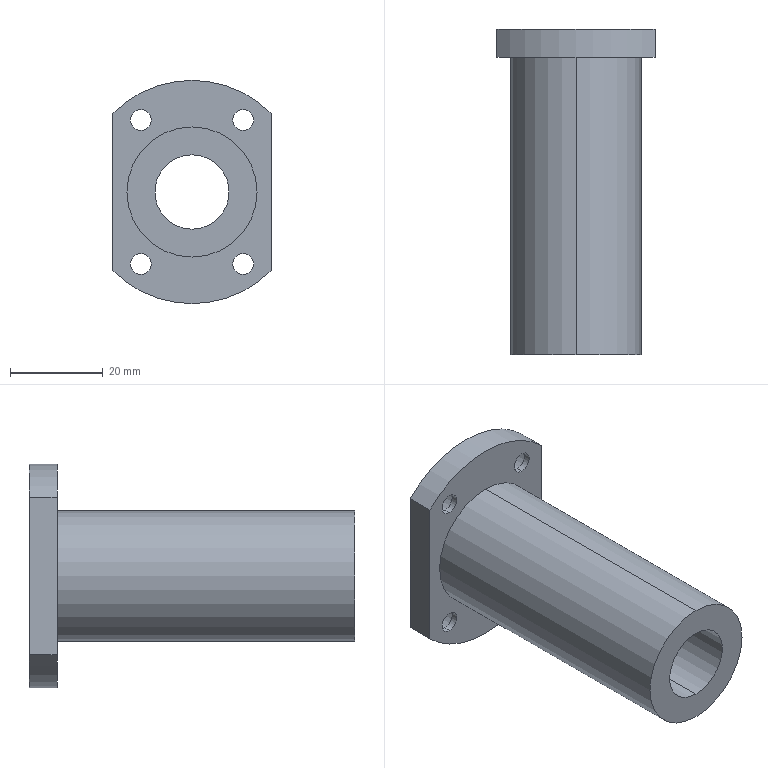Part | SolidWorks | features ICE 3, Extrusion 1, HoleWzd 1 | 1 solid | 32 faces | box 34 x 70 x 48 mm | volume 33217 mm3 | cylinder 23 | plane 9 | commonest cylinder face diameters 4.5 x8 8 x8 48 x3 16 x2 28 x2
STEP:
#1=CARTESIAN_POINT('',(11.,65.4,11.5));
#2=VERTEX_POINT('',#1);
#3=CARTESIAN_POINT('',(11.,65.4,19.5));
#4=VERTEX_POINT('',#3);
#5=CARTESIAN_POINT('',(11.,65.4,15.5));
#6=DIRECTION('',(0.,1.,0.));
#7=DIRECTION('',(0.,0.,1.));
#8=AXIS2_PLACEMENT_3D('',#5,#6,#7);
#9=CIRCLE('',#8,4.);
#10=EDGE_CURVE('',#2,#4,#9,.T.);
#11=ORIENTED_EDGE('',*,*,#10,.F.);
#12=CARTESIAN_POINT('',(11.,70.,11.5));
#13=VERTEX_POINT('',#12);
#14=CARTESIAN_POINT('',(11.,70.,11.5));
#15=DIRECTION('',(0.,1.,0.));
#16=VECTOR('',#15,1000.);
#17=LINE('',#14,#16);
#18=EDGE_CURVE('',#2,#13,#17,.T.);
#19=ORIENTED_EDGE('',*,*,#18,.T.);
#20=CARTESIAN_POINT('',(11.,70.,19.5));
#21=VERTEX_POINT('',#20);
#22=CARTESIAN_POINT('',(11.,70.,15.5));
#23=DIRECTION('',(0.,1.,0.));
#24=DIRECTION('',(0.,0.,1.));
#25=AXIS2_PLACEMENT_3D('',#22,#23,#24);
#26=CIRCLE('',#25,4.);
#27=EDGE_CURVE('',#13,#21,#26,.T.);
#28=ORIENTED_EDGE('',*,*,#27,.T.);
#29=CARTESIAN_POINT('',(11.,70.,19.5));
#30=DIRECTION('',(0.,1.,0.));
#31=VECTOR('',#30,1000.);
#32=LINE('',#29,#31);
#33=EDGE_CURVE('',#4,#21,#32,.T.);
#34=ORIENTED_EDGE('',*,*,#33,.F.);
#35=EDGE_LOOP('',(#11,#19,#28,#34));
#36=FACE_OUTER_BOUND('',#35,.T.);
#37=CARTESIAN_POINT('',(11.,70.,15.5));
#38=DIRECTION('',(0.,1.,0.));
#39=DIRECTION('',(0.,0.,1.));
#40=AXIS2_PLACEMENT_3D('',#37,#38,#39);
#41=CYLINDRICAL_SURFACE('',#40,4.);
#42=ADVANCED_FACE('',(#36),#41,.F.);
#43=CARTESIAN_POINT('',(11.,64.,13.25));
#44=VERTEX_POINT('',#43);
#45=CARTESIAN_POINT('',(11.,64.,17.75));
#46=VERTEX_POINT('',#45);
#47=CARTESIAN_POINT('',(11.,64.,15.5));
#48=DIRECTION('',(0.,1.,0.));
#49=DIRECTION('',(0.,0.,1.));
#50=AXIS2_PLACEMENT_3D('',#47,#48,#49);
#51=CIRCLE('',#50,2.25);
#52=EDGE_CURVE('',#44,#46,#51,.T.);
#53=ORIENTED_EDGE('',*,*,#52,.F.);
#54=CARTESIAN_POINT('',(11.,65.4,13.25));
#55=VERTEX_POINT('',#54);
#56=CARTESIAN_POINT('',(11.,70.,13.25));
#57=DIRECTION('',(0.,1.,0.));
#58=VECTOR('',#57,1000.);
#59=LINE('',#56,#58);
#60=EDGE_CURVE('',#44,#55,#59,.T.);
#61=ORIENTED_EDGE('',*,*,#60,.T.);
#62=CARTESIAN_POINT('',(11.,65.4,17.75));
#63=VERTEX_POINT('',#62);
#64=CARTESIAN_POINT('',(11.,65.4,15.5));
#65=DIRECTION('',(0.,1.,0.));
#66=DIRECTION('',(0.,0.,1.));
#67=AXIS2_PLACEMENT_3D('',#64,#65,#66);
#68=CIRCLE('',#67,2.25);
#69=EDGE_CURVE('',#55,#63,#68,.T.);
#70=ORIENTED_EDGE('',*,*,#69,.T.);
#71=CARTESIAN_POINT('',(11.,70.,17.75));
#72=DIRECTION('',(0.,1.,0.));
#73=VECTOR('',#72,1000.);
#74=LINE('',#71,#73);
#75=EDGE_CURVE('',#46,#63,#74,.T.);
#76=ORIENTED_EDGE('',*,*,#75,.F.);
#77=EDGE_LOOP('',(#53,#61,#70,#76));
#78=FACE_OUTER_BOUND('',#77,.T.);
#79=CARTESIAN_POINT('',(11.,70.,15.5));
#80=DIRECTION('',(0.,1.,0.));
#81=DIRECTION('',(0.,0.,1.));
#82=AXIS2_PLACEMENT_3D('',#79,#80,#81);
#83=CYLINDRICAL_SURFACE('',#82,2.25);
#84=ADVANCED_FACE('',(#78),#83,.F.);
#85=CARTESIAN_POINT('',(-11.,65.4,11.5));
#86=VERTEX_POINT('',#85);
#87=CARTESIAN_POINT('',(-11.,65.4,19.5));
#88=VERTEX_POINT('',#87);
#89=CARTESIAN_POINT('',(-11.,65.4,15.5));
#90=DIRECTION('',(0.,1.,0.));
#91=DIRECTION('',(0.,0.,1.));
#92=AXIS2_PLACEMENT_3D('',#89,#90,#91);
#93=CIRCLE('',#92,4.);
#94=EDGE_CURVE('',#86,#88,#93,.T.);
#95=ORIENTED_EDGE('',*,*,#94,.F.);
#96=CARTESIAN_POINT('',(-11.,70.,11.5));
#97=VERTEX_POINT('',#96);
#98=CARTESIAN_POINT('',(-11.,70.,11.5));
#99=DIRECTION('',(0.,1.,0.));
#100=VECTOR('',#99,1000.);
#101=LINE('',#98,#100);
#102=EDGE_CURVE('',#86,#97,#101,.T.);
#103=ORIENTED_EDGE('',*,*,#102,.T.);
#104=CARTESIAN_POINT('',(-11.,70.,19.5));
#105=VERTEX_POINT('',#104);
#106=CARTESIAN_POINT('',(-11.,70.,15.5));
#107=DIRECTION('',(0.,1.,0.));
#108=DIRECTION('',(0.,0.,1.));
#109=AXIS2_PLACEMENT_3D('',#106,#107,#108);
#110=CIRCLE('',#109,4.);
#111=EDGE_CURVE('',#97,#105,#110,.T.);
#112=ORIENTED_EDGE('',*,*,#111,.T.);
#113=CARTESIAN_POINT('',(-11.,70.,19.5));
#114=DIRECTION('',(0.,1.,0.));
#115=VECTOR('',#114,1000.);
#116=LINE('',#113,#115);
#117=EDGE_CURVE('',#88,#105,#116,.T.);
#118=ORIENTED_EDGE('',*,*,#117,.F.);
#119=EDGE_LOOP('',(#95,#103,#112,#118));
#120=FACE_OUTER_BOUND('',#119,.T.);
#121=CARTESIAN_POINT('',(-11.,70.,15.5));
#122=DIRECTION('',(0.,1.,0.));
#123=DIRECTION('',(0.,0.,1.));
#124=AXIS2_PLACEMENT_3D('',#121,#122,#123);
#125=CYLINDRICAL_SURFACE('',#124,4.);
#126=ADVANCED_FACE('',(#120),#125,.F.);
#127=CARTESIAN_POINT('',(-11.,64.,13.25));
#128=VERTEX_POINT('',#127);
#129=CARTESIAN_POINT('',(-11.,64.,17.75));
#130=VERTEX_POINT('',#129);
#131=CARTESIAN_POINT('',(-11.,64.,15.5));
#132=DIRECTION('',(0.,1.,0.));
#133=DIRECTION('',(0.,0.,1.));
#134=AXIS2_PLACEMENT_3D('',#131,#132,#133);
#135=CIRCLE('',#134,2.25);
#136=EDGE_CURVE('',#128,#130,#135,.T.);
#137=ORIENTED_EDGE('',*,*,#136,.F.);
#138=CARTESIAN_POINT('',(-11.,65.4,13.25));
#139=VERTEX_POINT('',#138);
#140=CARTESIAN_POINT('',(-11.,70.,13.25));
#141=DIRECTION('',(0.,1.,0.));
#142=VECTOR('',#141,1000.);
#143=LINE('',#140,#142);
#144=EDGE_CURVE('',#128,#139,#143,.T.);
#145=ORIENTED_EDGE('',*,*,#144,.T.);
#146=CARTESIAN_POINT('',(-11.,65.4,17.75));
#147=VERTEX_POINT('',#146);
#148=CARTESIAN_POINT('',(-11.,65.4,15.5));
#149=DIRECTION('',(0.,1.,0.));
#150=DIRECTION('',(0.,0.,1.));
#151=AXIS2_PLACEMENT_3D('',#148,#149,#150);
#152=CIRCLE('',#151,2.25);
#153=EDGE_CURVE('',#139,#147,#152,.T.);
#154=ORIENTED_EDGE('',*,*,#153,.T.);
#155=CARTESIAN_POINT('',(-11.,70.,17.75));
#156=DIRECTION('',(0.,1.,0.));
#157=VECTOR('',#156,1000.);
#158=LINE('',#155,#157);
#159=EDGE_CURVE('',#130,#147,#158,.T.);
#160=ORIENTED_EDGE('',*,*,#159,.F.);
#161=EDGE_LOOP('',(#137,#145,#154,#160));
#162=FACE_OUTER_BOUND('',#161,.T.);
#163=CARTESIAN_POINT('',(-11.,70.,15.5));
#164=DIRECTION('',(0.,1.,0.));
#165=DIRECTION('',(0.,0.,1.));
#166=AXIS2_PLACEMENT_3D('',#163,#164,#165);
#167=CYLINDRICAL_SURFACE('',#166,2.25);
#168=ADVANCED_FACE('',(#162),#167,.F.);
#169=CARTESIAN_POINT('',(-11.,65.4,-19.5));
#170=VERTEX_POINT('',#169);
#171=CARTESIAN_POINT('',(-11.,65.4,-11.5));
#172=VERTEX_POINT('',#171);
#173=CARTESIAN_POINT('',(-11.,65.4,-15.5));
#174=DIRECTION('',(0.,1.,0.));
#175=DIRECTION('',(0.,0.,1.));
#176=AXIS2_PLACEMENT_3D('',#173,#174,#175);
#177=CIRCLE('',#176,4.);
#178=EDGE_CURVE('',#170,#172,#177,.T.);
#179=ORIENTED_EDGE('',*,*,#178,.F.);
#180=CARTESIAN_POINT('',(-11.,70.,-19.5));
#181=VERTEX_POINT('',#180);
#182=CARTESIAN_POINT('',(-11.,70.,-19.5));
#183=DIRECTION('',(0.,1.,0.));
#184=VECTOR('',#183,1000.);
#185=LINE('',#182,#184);
#186=EDGE_CURVE('',#170,#181,#185,.T.);
#187=ORIENTED_EDGE('',*,*,#186,.T.);
#188=CARTESIAN_POINT('',(-11.,70.,-11.5));
#189=VERTEX_POINT('',#188);
#190=CARTESIAN_POINT('',(-11.,70.,-15.5));
#191=DIRECTION('',(0.,1.,0.));
#192=DIRECTION('',(0.,0.,1.));
#193=AXIS2_PLACEMENT_3D('',#190,#191,#192);
#194=CIRCLE('',#193,4.);
#195=EDGE_CURVE('',#181,#189,#194,.T.);
#196=ORIENTED_EDGE('',*,*,#195,.T.);
#197=CARTESIAN_POINT('',(-11.,70.,-11.5));
#198=DIRECTION('',(0.,1.,0.));
#199=VECTOR('',#198,1000.);
#200=LINE('',#197,#199);
#201=EDGE_CURVE('',#172,#189,#200,.T.);
#202=ORIENTED_EDGE('',*,*,#201,.F.);
#203=EDGE_LOOP('',(#179,#187,#196,#202));
#204=FACE_OUTER_BOUND('',#203,.T.);
#205=CARTESIAN_POINT('',(-11.,70.,-15.5));
#206=DIRECTION('',(0.,1.,0.));
#207=DIRECTION('',(0.,0.,1.));
#208=AXIS2_PLACEMENT_3D('',#205,#206,#207);
#209=CYLINDRICAL_SURFACE('',#208,4.);
#210=ADVANCED_FACE('',(#204),#209,.F.);
#211=CARTESIAN_POINT('',(-11.,64.,-17.75));
#212=VERTEX_POINT('',#211);
#213=CARTESIAN_POINT('',(-11.,64.,-13.25));
#214=VERTEX_POINT('',#213);
#215=CARTESIAN_POINT('',(-11.,64.,-15.5));
#216=DIRECTION('',(0.,1.,0.));
#217=DIRECTION('',(0.,0.,1.));
#218=AXIS2_PLACEMENT_3D('',#215,#216,#217);
#219=CIRCLE('',#218,2.25);
#220=EDGE_CURVE('',#212,#214,#219,.T.);
#221=ORIENTED_EDGE('',*,*,#220,.F.);
#222=CARTESIAN_POINT('',(-11.,65.4,-17.75));
#223=VERTEX_POINT('',#222);
#224=CARTESIAN_POINT('',(-11.,70.,-17.75));
#225=DIRECTION('',(0.,1.,0.));
#226=VECTOR('',#225,1000.);
#227=LINE('',#224,#226);
#228=EDGE_CURVE('',#212,#223,#227,.T.);
#229=ORIENTED_EDGE('',*,*,#228,.T.);
#230=CARTESIAN_POINT('',(-11.,65.4,-13.25));
#231=VERTEX_POINT('',#230);
#232=CARTESIAN_POINT('',(-11.,65.4,-15.5));
#233=DIRECTION('',(0.,1.,0.));
#234=DIRECTION('',(0.,0.,1.));
#235=AXIS2_PLACEMENT_3D('',#232,#233,#234);
#236=CIRCLE('',#235,2.25);
#237=EDGE_CURVE('',#223,#231,#236,.T.);
#238=ORIENTED_EDGE('',*,*,#237,.T.);
#239=CARTESIAN_POINT('',(-11.,70.,-13.25));
#240=DIRECTION('',(0.,1.,0.));
#241=VECTOR('',#240,1000.);
#242=LINE('',#239,#241);
#243=EDGE_CURVE('',#214,#231,#242,.T.);
#244=ORIENTED_EDGE('',*,*,#243,.F.);
#245=EDGE_LOOP('',(#221,#229,#238,#244));
#246=FACE_OUTER_BOUND('',#245,.T.);
#247=CARTESIAN_POINT('',(-11.,70.,-15.5));
#248=DIRECTION('',(0.,1.,0.));
#249=DIRECTION('',(0.,0.,1.));
#250=AXIS2_PLACEMENT_3D('',#247,#248,#249);
#251=CYLINDRICAL_SURFACE('',#250,2.25);
#252=ADVANCED_FACE('',(#246),#251,.F.);
#253=CARTESIAN_POINT('',(11.,65.4,-19.5));
#254=VERTEX_POINT('',#253);
#255=CARTESIAN_POINT('',(11.,65.4,-11.5));
#256=VERTEX_POINT('',#255);
#257=CARTESIAN_POINT('',(11.,65.4,-15.5));
#258=DIRECTION('',(0.,1.,0.));
#259=DIRECTION('',(0.,0.,1.));
#260=AXIS2_PLACEMENT_3D('',#257,#258,#259);
#261=CIRCLE('',#260,4.);
#262=EDGE_CURVE('',#254,#256,#261,.T.);
#263=ORIENTED_EDGE('',*,*,#262,.F.);
#264=CARTESIAN_POINT('',(11.,70.,-19.5));
#265=VERTEX_POINT('',#264);
#266=CARTESIAN_POINT('',(11.,70.,-19.5));
#267=DIRECTION('',(0.,1.,0.));
#268=VECTOR('',#267,1000.);
#269=LINE('',#266,#268);
#270=EDGE_CURVE('',#254,#265,#269,.T.);
#271=ORIENTED_EDGE('',*,*,#270,.T.);
#272=CARTESIAN_POINT('',(11.,70.,-11.5));
#273=VERTEX_POINT('',#272);
#274=CARTESIAN_POINT('',(11.,70.,-15.5));
#275=DIRECTION('',(0.,1.,0.));
#276=DIRECTION('',(0.,0.,1.));
#277=AXIS2_PLACEMENT_3D('',#274,#275,#276);
#278=CIRCLE('',#277,4.);
#279=EDGE_CURVE('',#265,#273,#278,.T.);
#280=ORIENTED_EDGE('',*,*,#279,.T.);
#281=CARTESIAN_POINT('',(11.,70.,-11.5));
#282=DIRECTION('',(0.,1.,0.));
#283=VECTOR('',#282,1000.);
#284=LINE('',#281,#283);
#285=EDGE_CURVE('',#256,#273,#284,.T.);
#286=ORIENTED_EDGE('',*,*,#285,.F.);
#287=EDGE_LOOP('',(#263,#271,#280,#286));
#288=FACE_OUTER_BOUND('',#287,.T.);
#289=CARTESIAN_POINT('',(11.,70.,-15.5));
#290=DIRECTION('',(0.,1.,0.));
#291=DIRECTION('',(0.,0.,1.));
#292=AXIS2_PLACEMENT_3D('',#289,#290,#291);
#293=CYLINDRICAL_SURFACE('',#292,4.);
#294=ADVANCED_FACE('',(#288),#293,.F.);
#295=CARTESIAN_POINT('',(11.,64.,-17.75));
#296=VERTEX_POINT('',#295);
#297=CARTESIAN_POINT('',(11.,64.,-13.25));
#298=VERTEX_POINT('',#297);
#299=CARTESIAN_POINT('',(11.,64.,-15.5));
#300=DIRECTION('',(0.,1.,0.));
#301=DIRECTION('',(0.,0.,1.));
#302=AXIS2_PLACEMENT_3D('',#299,#300,#301);
#303=CIRCLE('',#302,2.25);
#304=EDGE_CURVE('',#296,#298,#303,.T.);
#305=ORIENTED_EDGE('',*,*,#304,.F.);
#306=CARTESIAN_POINT('',(11.,65.4,-17.75));
#307=VERTEX_POINT('',#306);
#308=CARTESIAN_POINT('',(11.,70.,-17.75));
#309=DIRECTION('',(0.,1.,0.));
#310=VECTOR('',#309,1000.);
#311=LINE('',#308,#310);
#312=EDGE_CURVE('',#296,#307,#311,.T.);
#313=ORIENTED_EDGE('',*,*,#312,.T.);
#314=CARTESIAN_POINT('',(11.,65.4,-13.25));
#315=VERTEX_POINT('',#314);
#316=CARTESIAN_POINT('',(11.,65.4,-15.5));
#317=DIRECTION('',(0.,1.,0.));
#318=DIRECTION('',(0.,0.,1.));
#319=AXIS2_PLACEMENT_3D('',#316,#317,#318);
#320=CIRCLE('',#319,2.25);
#321=EDGE_CURVE('',#307,#315,#320,.T.);
#322=ORIENTED_EDGE('',*,*,#321,.T.);
#323=CARTESIAN_POINT('',(11.,70.,-13.25));
#324=DIRECTION('',(0.,1.,0.));
#325=VECTOR('',#324,1000.);
#326=LINE('',#323,#325);
#327=EDGE_CURVE('',#298,#315,#326,.T.);
#328=ORIENTED_EDGE('',*,*,#327,.F.);
#329=EDGE_LOOP('',(#305,#313,#322,#328));
#330=FACE_OUTER_BOUND('',#329,.T.);
#331=CARTESIAN_POINT('',(11.,70.,-15.5));
#332=DIRECTION('',(0.,1.,0.));
#333=DIRECTION('',(0.,0.,1.));
#334=AXIS2_PLACEMENT_3D('',#331,#332,#333);
#335=CYLINDRICAL_SURFACE('',#334,2.25);
#336=ADVANCED_FACE('',(#330),#335,.F.);
#337=CARTESIAN_POINT('',(0.,70.,8.));
#338=VERTEX_POINT('',#337);
#339=CARTESIAN_POINT('',(0.,70.,-8.));
#340=VERTEX_POINT('',#339);
#341=CARTESIAN_POINT('',(0.,70.,0.));
#342=DIRECTION('',(0.,-1.,0.));
#343=DIRECTION('',(0.,0.,-1.));
#344=AXIS2_PLACEMENT_3D('',#341,#342,#343);
#345=CIRCLE('',#344,8.);
#346=EDGE_CURVE('',#338,#340,#345,.T.);
#347=ORIENTED_EDGE('',*,*,#346,.F.);
#348=CARTESIAN_POINT('',(0.,0.,8.));
#349=VERTEX_POINT('',#348);
#350=CARTESIAN_POINT('',(0.,70.,8.));
#351=DIRECTION('',(0.,-1.,0.));
#352=VECTOR('',#351,1000.);
#353=LINE('',#350,#352);
#354=EDGE_CURVE('',#338,#349,#353,.T.);
#355=ORIENTED_EDGE('',*,*,#354,.T.);
#356=CARTESIAN_POINT('',(0.,0.,-8.));
#357=VERTEX_POINT('',#356);
#358=CARTESIAN_POINT('',(0.,0.,0.));
#359=DIRECTION('',(0.,-1.,0.));
#360=DIRECTION('',(0.,0.,-1.));
#361=AXIS2_PLACEMENT_3D('',#358,#359,#360);
#362=CIRCLE('',#361,8.);
#363=EDGE_CURVE('',#349,#357,#362,.T.);
#364=ORIENTED_EDGE('',*,*,#363,.T.);
#365=CARTESIAN_POINT('',(0.,70.,-8.));
#366=DIRECTION('',(0.,-1.,0.));
#367=VECTOR('',#366,1000.);
#368=LINE('',#365,#367);
#369=EDGE_CURVE('',#340,#357,#368,.T.);
#370=ORIENTED_EDGE('',*,*,#369,.F.);
#371=EDGE_LOOP('',(#347,#355,#364,#370));
#372=FACE_OUTER_BOUND('',#371,.T.);
#373=CARTESIAN_POINT('',(0.,70.,0.));
#374=DIRECTION('',(0.,-1.,0.));
#375=DIRECTION('',(0.,0.,-1.));
#376=AXIS2_PLACEMENT_3D('',#373,#374,#375);
#377=CYLINDRICAL_SURFACE('',#376,8.);
#378=ADVANCED_FACE('',(#372),#377,.F.);
#379=CARTESIAN_POINT('',(0.,64.,14.));
#380=VERTEX_POINT('',#379);
#381=CARTESIAN_POINT('',(0.,64.,-14.));
#382=VERTEX_POINT('',#381);
#383=CARTESIAN_POINT('',(0.,64.,0.));
#384=DIRECTION('',(0.,1.,0.));
#385=DIRECTION('',(0.,0.,1.));
#386=AXIS2_PLACEMENT_3D('',#383,#384,#385);
#387=CIRCLE('',#386,14.);
#388=EDGE_CURVE('',#380,#382,#387,.T.);
#389=ORIENTED_EDGE('',*,*,#388,.F.);
#390=CARTESIAN_POINT('',(0.,0.,14.));
#391=VERTEX_POINT('',#390);
#392=CARTESIAN_POINT('',(0.,64.,14.));
#393=DIRECTION('',(0.,-1.,0.));
#394=VECTOR('',#393,1000.);
#395=LINE('',#392,#394);
#396=EDGE_CURVE('',#380,#391,#395,.T.);
#397=ORIENTED_EDGE('',*,*,#396,.T.);
#398=CARTESIAN_POINT('',(0.,0.,-14.));
#399=VERTEX_POINT('',#398);
#400=CARTESIAN_POINT('',(0.,0.,0.));
#401=DIRECTION('',(0.,1.,0.));
#402=DIRECTION('',(0.,0.,1.));
#403=AXIS2_PLACEMENT_3D('',#400,#401,#402);
#404=CIRCLE('',#403,14.);
#405=EDGE_CURVE('',#391,#399,#404,.T.);
#406=ORIENTED_EDGE('',*,*,#405,.T.);
#407=CARTESIAN_POINT('',(0.,64.,-14.));
#408=DIRECTION('',(0.,-1.,0.));
#409=VECTOR('',#408,1000.);
#410=LINE('',#407,#409);
#411=EDGE_CURVE('',#382,#399,#410,.T.);
#412=ORIENTED_EDGE('',*,*,#411,.F.);
#413=EDGE_LOOP('',(#389,#397,#406,#412));
#414=FACE_OUTER_BOUND('',#413,.T.);
#415=CARTESIAN_POINT('',(0.,64.,0.));
#416=DIRECTION('',(0.,-1.,0.));
#417=DIRECTION('',(0.,0.,-1.));
#418=AXIS2_PLACEMENT_3D('',#415,#416,#417);
#419=CYLINDRICAL_SURFACE('',#418,14.);
#420=ADVANCED_FACE('',(#414),#419,.T.);
#421=CARTESIAN_POINT('',(0.,70.,-24.));
#422=VERTEX_POINT('',#421);
#423=CARTESIAN_POINT('',(-17.,70.,-16.941));
#424=VERTEX_POINT('',#423);
#425=CARTESIAN_POINT('',(0.,70.,0.));
#426=DIRECTION('',(0.,1.,0.));
#427=DIRECTION('',(0.,0.,1.));
#428=AXIS2_PLACEMENT_3D('',#425,#426,#427);
#429=CIRCLE('',#428,24.);
#430=EDGE_CURVE('',#422,#424,#429,.T.);
#431=ORIENTED_EDGE('',*,*,#430,.F.);
#432=CARTESIAN_POINT('',(0.,64.,-24.));
#433=VERTEX_POINT('',#432);
#434=CARTESIAN_POINT('',(0.,70.,-24.));
#435=DIRECTION('',(0.,-1.,0.));
#436=VECTOR('',#435,1000.);
#437=LINE('',#434,#436);
#438=EDGE_CURVE('',#422,#433,#437,.T.);
#439=ORIENTED_EDGE('',*,*,#438,.T.);
#440=CARTESIAN_POINT('',(-17.,64.,-16.941));
#441=VERTEX_POINT('',#440);
#442=CARTESIAN_POINT('',(0.,64.,0.));
#443=DIRECTION('',(0.,1.,0.));
#444=DIRECTION('',(0.,0.,1.));
#445=AXIS2_PLACEMENT_3D('',#442,#443,#444);
#446=CIRCLE('',#445,24.);
#447=EDGE_CURVE('',#433,#441,#446,.T.);
#448=ORIENTED_EDGE('',*,*,#447,.T.);
#449=CARTESIAN_POINT('',(-17.,64.,-16.941));
#450=DIRECTION('',(0.,1.,0.));
#451=VECTOR('',#450,1000.);
#452=LINE('',#449,#451);
#453=EDGE_CURVE('',#441,#424,#452,.T.);
#454=ORIENTED_EDGE('',*,*,#453,.T.);
#455=EDGE_LOOP('',(#431,#439,#448,#454));
#456=FACE_OUTER_BOUND('',#455,.T.);
#457=CARTESIAN_POINT('',(0.,70.,0.));
#458=DIRECTION('',(0.,-1.,0.));
#459=DIRECTION('',(0.,0.,-1.));
#460=AXIS2_PLACEMENT_3D('',#457,#458,#459);
#461=CYLINDRICAL_SURFACE('',#460,24.);
#462=ADVANCED_FACE('',(#456),#461,.T.);
#463=CARTESIAN_POINT('',(11.,64.,15.5));
#464=DIRECTION('',(0.,1.,0.));
#465=DIRECTION('',(0.,0.,1.));
#466=AXIS2_PLACEMENT_3D('',#463,#464,#465);
#467=CIRCLE('',#466,2.25);
#468=EDGE_CURVE('',#46,#44,#467,.T.);
#469=ORIENTED_EDGE('',*,*,#468,.T.);
#470=ORIENTED_EDGE('',*,*,#52,.T.);
#471=EDGE_LOOP('',(#469,#470));
#472=FACE_BOUND('',#471,.T.);
#473=CARTESIAN_POINT('',(-11.,64.,15.5));
#474=DIRECTION('',(0.,1.,0.));
#475=DIRECTION('',(0.,0.,1.));
#476=AXIS2_PLACEMENT_3D('',#473,#474,#475);
#477=CIRCLE('',#476,2.25);
#478=EDGE_CURVE('',#130,#128,#477,.T.);
#479=ORIENTED_EDGE('',*,*,#478,.T.);
#480=ORIENTED_EDGE('',*,*,#136,.T.);
#481=EDGE_LOOP('',(#479,#480));
#482=FACE_BOUND('',#481,.T.);
#483=CARTESIAN_POINT('',(-11.,64.,-15.5));
#484=DIRECTION('',(0.,1.,0.));
#485=DIRECTION('',(0.,0.,1.));
#486=AXIS2_PLACEMENT_3D('',#483,#484,#485);
#487=CIRCLE('',#486,2.25);
#488=EDGE_CURVE('',#214,#212,#487,.T.);
#489=ORIENTED_EDGE('',*,*,#488,.T.);
#490=ORIENTED_EDGE('',*,*,#220,.T.);
#491=EDGE_LOOP('',(#489,#490));
#492=FACE_BOUND('',#491,.T.);
#493=CARTESIAN_POINT('',(11.,64.,-15.5));
#494=DIRECTION('',(0.,1.,0.));
#495=DIRECTION('',(0.,0.,1.));
#496=AXIS2_PLACEMENT_3D('',#493,#494,#495);
#497=CIRCLE('',#496,2.25);
#498=EDGE_CURVE('',#298,#296,#497,.T.);
#499=ORIENTED_EDGE('',*,*,#498,.T.);
#500=ORIENTED_EDGE('',*,*,#304,.T.);
#501=EDGE_LOOP('',(#499,#500));
#502=FACE_BOUND('',#501,.T.);
#503=CARTESIAN_POINT('',(0.,64.,0.));
#504=DIRECTION('',(0.,1.,0.));
#505=DIRECTION('',(0.,0.,1.));
#506=AXIS2_PLACEMENT_3D('',#503,#504,#505);
#507=CIRCLE('',#506,14.);
#508=EDGE_CURVE('',#382,#380,#507,.T.);
#509=ORIENTED_EDGE('',*,*,#508,.T.);
#510=ORIENTED_EDGE('',*,*,#388,.T.);
#511=EDGE_LOOP('',(#509,#510));
#512=FACE_BOUND('',#511,.T.);
#513=CARTESIAN_POINT('',(17.,64.,16.941));
#514=VERTEX_POINT('',#513);
#515=CARTESIAN_POINT('',(17.,64.,-16.941));
#516=VERTEX_POINT('',#515);
#517=CARTESIAN_POINT('',(17.,64.,-16.941));
#518=DIRECTION('',(0.,0.,-1.));
#519=VECTOR('',#518,1000.);
#520=LINE('',#517,#519);
#521=EDGE_CURVE('',#514,#516,#520,.T.);
#522=ORIENTED_EDGE('',*,*,#521,.F.);
#523=CARTESIAN_POINT('',(-17.,64.,16.941));
#524=VERTEX_POINT('',#523);
#525=CARTESIAN_POINT('',(0.,64.,0.));
#526=DIRECTION('',(0.,1.,0.));
#527=DIRECTION('',(0.,0.,1.));
#528=AXIS2_PLACEMENT_3D('',#525,#526,#527);
#529=CIRCLE('',#528,24.);
#530=EDGE_CURVE('',#524,#514,#529,.T.);
#531=ORIENTED_EDGE('',*,*,#530,.F.);
#532=CARTESIAN_POINT('',(-17.,64.,-16.941));
#533=DIRECTION('',(0.,0.,1.));
#534=VECTOR('',#533,1000.);
#535=LINE('',#532,#534);
#536=EDGE_CURVE('',#441,#524,#535,.T.);
#537=ORIENTED_EDGE('',*,*,#536,.F.);
#538=ORIENTED_EDGE('',*,*,#447,.F.);
#539=CARTESIAN_POINT('',(0.,64.,0.));
#540=DIRECTION('',(0.,1.,0.));
#541=DIRECTION('',(0.,0.,1.));
#542=AXIS2_PLACEMENT_3D('',#539,#540,#541);
#543=CIRCLE('',#542,24.);
#544=EDGE_CURVE('',#516,#433,#543,.T.);
#545=ORIENTED_EDGE('',*,*,#544,.F.);
#546=EDGE_LOOP('',(#522,#531,#537,#538,#545));
#547=FACE_OUTER_BOUND('',#546,.T.);
#548=CARTESIAN_POINT('',(0.,64.,0.));
#549=DIRECTION('',(0.,1.,0.));
#550=DIRECTION('',(0.,0.,1.));
#551=AXIS2_PLACEMENT_3D('',#548,#549,#550);
#552=PLANE('',#551);
#553=ADVANCED_FACE('',(#472,#482,#492,#502,#512,#547),#552,.F.);
#554=CARTESIAN_POINT('',(17.,70.,16.941));
#555=VERTEX_POINT('',#554);
#556=CARTESIAN_POINT('',(17.,64.,16.941));
#557=DIRECTION('',(0.,1.,0.));
#558=VECTOR('',#557,1000.);
#559=LINE('',#556,#558);
#560=EDGE_CURVE('',#514,#555,#559,.T.);
#561=ORIENTED_EDGE('',*,*,#560,.T.);
#562=CARTESIAN_POINT('',(-17.,70.,16.941));
#563=VERTEX_POINT('',#562);
#564=CARTESIAN_POINT('',(0.,70.,0.));
#565=DIRECTION('',(0.,1.,0.));
#566=DIRECTION('',(0.,0.,1.));
#567=AXIS2_PLACEMENT_3D('',#564,#565,#566);
#568=CIRCLE('',#567,24.);
#569=EDGE_CURVE('',#563,#555,#568,.T.);
#570=ORIENTED_EDGE('',*,*,#569,.F.);
#571=CARTESIAN_POINT('',(-17.,64.,16.941));
#572=DIRECTION('',(0.,1.,0.));
#573=VECTOR('',#572,1000.);
#574=LINE('',#571,#573);
#575=EDGE_CURVE('',#524,#563,#574,.T.);
#576=ORIENTED_EDGE('',*,*,#575,.F.);
#577=ORIENTED_EDGE('',*,*,#530,.T.);
#578=EDGE_LOOP('',(#561,#570,#576,#577));
#579=FACE_OUTER_BOUND('',#578,.T.);
#580=CARTESIAN_POINT('',(0.,70.,0.));
#581=DIRECTION('',(0.,-1.,0.));
#582=DIRECTION('',(0.,0.,-1.));
#583=AXIS2_PLACEMENT_3D('',#580,#581,#582);
#584=CYLINDRICAL_SURFACE('',#583,24.);
#585=ADVANCED_FACE('',(#579),#584,.T.);
#586=ORIENTED_EDGE('',*,*,#438,.F.);
#587=CARTESIAN_POINT('',(17.,70.,-16.941));
#588=VERTEX_POINT('',#587);
#589=CARTESIAN_POINT('',(0.,70.,0.));
#590=DIRECTION('',(0.,1.,0.));
#591=DIRECTION('',(0.,0.,1.));
#592=AXIS2_PLACEMENT_3D('',#589,#590,#591);
#593=CIRCLE('',#592,24.);
#594=EDGE_CURVE('',#588,#422,#593,.T.);
#595=ORIENTED_EDGE('',*,*,#594,.F.);
#596=CARTESIAN_POINT('',(17.,64.,-16.941));
#597=DIRECTION('',(0.,1.,0.));
#598=VECTOR('',#597,1000.);
#599=LINE('',#596,#598);
#600=EDGE_CURVE('',#516,#588,#599,.T.);
#601=ORIENTED_EDGE('',*,*,#600,.F.);
#602=ORIENTED_EDGE('',*,*,#544,.T.);
#603=EDGE_LOOP('',(#586,#595,#601,#602));
#604=FACE_OUTER_BOUND('',#603,.T.);
#605=CARTESIAN_POINT('',(0.,70.,0.));
#606=DIRECTION('',(0.,-1.,0.));
#607=DIRECTION('',(0.,0.,-1.));
#608=AXIS2_PLACEMENT_3D('',#605,#606,#607);
#609=CYLINDRICAL_SURFACE('',#608,24.);
#610=ADVANCED_FACE('',(#604),#609,.T.);
#611=CARTESIAN_POINT('',(11.,70.,15.5));
#612=DIRECTION('',(0.,1.,0.));
#613=DIRECTION('',(0.,0.,1.));
#614=AXIS2_PLACEMENT_3D('',#611,#612,#613);
#615=CIRCLE('',#614,4.);
#616=EDGE_CURVE('',#21,#13,#615,.T.);
#617=ORIENTED_EDGE('',*,*,#616,.F.);
#618=ORIENTED_EDGE('',*,*,#27,.F.);
#619=EDGE_LOOP('',(#617,#618));
#620=FACE_BOUND('',#619,.T.);
#621=CARTESIAN_POINT('',(-11.,70.,15.5));
#622=DIRECTION('',(0.,1.,0.));
#623=DIRECTION('',(0.,0.,1.));
#624=AXIS2_PLACEMENT_3D('',#621,#622,#623);
#625=CIRCLE('',#624,4.);
#626=EDGE_CURVE('',#105,#97,#625,.T.);
#627=ORIENTED_EDGE('',*,*,#626,.F.);
#628=ORIENTED_EDGE('',*,*,#111,.F.);
#629=EDGE_LOOP('',(#627,#628));
#630=FACE_BOUND('',#629,.T.);
#631=CARTESIAN_POINT('',(-11.,70.,-15.5));
#632=DIRECTION('',(0.,1.,0.));
#633=DIRECTION('',(0.,0.,1.));
#634=AXIS2_PLACEMENT_3D('',#631,#632,#633);
#635=CIRCLE('',#634,4.);
#636=EDGE_CURVE('',#189,#181,#635,.T.);
#637=ORIENTED_EDGE('',*,*,#636,.F.);
#638=ORIENTED_EDGE('',*,*,#195,.F.);
#639=EDGE_LOOP('',(#637,#638));
#640=FACE_BOUND('',#639,.T.);
#641=CARTESIAN_POINT('',(11.,70.,-15.5));
#642=DIRECTION('',(0.,1.,0.));
#643=DIRECTION('',(0.,0.,1.));
#644=AXIS2_PLACEMENT_3D('',#641,#642,#643);
#645=CIRCLE('',#644,4.);
#646=EDGE_CURVE('',#273,#265,#645,.T.);
#647=ORIENTED_EDGE('',*,*,#646,.F.);
#648=ORIENTED_EDGE('',*,*,#279,.F.);
#649=EDGE_LOOP('',(#647,#648));
#650=FACE_BOUND('',#649,.T.);
#651=CARTESIAN_POINT('',(0.,70.,0.));
#652=DIRECTION('',(0.,-1.,0.));
#653=DIRECTION('',(0.,0.,-1.));
#654=AXIS2_PLACEMENT_3D('',#651,#652,#653);
#655=CIRCLE('',#654,8.);
#656=EDGE_CURVE('',#340,#338,#655,.T.);
#657=ORIENTED_EDGE('',*,*,#656,.T.);
#658=ORIENTED_EDGE('',*,*,#346,.T.);
#659=EDGE_LOOP('',(#657,#658));
#660=FACE_BOUND('',#659,.T.);
#661=ORIENTED_EDGE('',*,*,#569,.T.);
#662=CARTESIAN_POINT('',(17.,70.,-16.941));
#663=DIRECTION('',(0.,0.,-1.));
#664=VECTOR('',#663,1000.);
#665=LINE('',#662,#664);
#666=EDGE_CURVE('',#555,#588,#665,.T.);
#667=ORIENTED_EDGE('',*,*,#666,.T.);
#668=ORIENTED_EDGE('',*,*,#594,.T.);
#669=ORIENTED_EDGE('',*,*,#430,.T.);
#670=CARTESIAN_POINT('',(-17.,70.,-16.941));
#671=DIRECTION('',(0.,0.,1.));
#672=VECTOR('',#671,1000.);
#673=LINE('',#670,#672);
#674=EDGE_CURVE('',#424,#563,#673,.T.);
#675=ORIENTED_EDGE('',*,*,#674,.T.);
#676=EDGE_LOOP('',(#661,#667,#668,#669,#675));
#677=FACE_OUTER_BOUND('',#676,.T.);
#678=CARTESIAN_POINT('',(0.,70.,0.));
#679=DIRECTION('',(0.,1.,0.));
#680=DIRECTION('',(0.,0.,1.));
#681=AXIS2_PLACEMENT_3D('',#678,#679,#680);
#682=PLANE('',#681);
#683=ADVANCED_FACE('',(#620,#630,#640,#650,#660,#677),#682,.T.);
#684=ORIENTED_EDGE('',*,*,#396,.F.);
#685=ORIENTED_EDGE('',*,*,#508,.F.);
#686=ORIENTED_EDGE('',*,*,#411,.T.);
#687=CARTESIAN_POINT('',(0.,0.,0.));
#688=DIRECTION('',(0.,1.,0.));
#689=DIRECTION('',(0.,0.,1.));
#690=AXIS2_PLACEMENT_3D('',#687,#688,#689);
#691=CIRCLE('',#690,14.);
#692=EDGE_CURVE('',#399,#391,#691,.T.);
#693=ORIENTED_EDGE('',*,*,#692,.T.);
#694=EDGE_LOOP('',(#684,#685,#686,#693));
#695=FACE_OUTER_BOUND('',#694,.T.);
#696=CARTESIAN_POINT('',(0.,64.,0.));
#697=DIRECTION('',(0.,-1.,0.));
#698=DIRECTION('',(0.,0.,-1.));
#699=AXIS2_PLACEMENT_3D('',#696,#697,#698);
#700=CYLINDRICAL_SURFACE('',#699,14.);
#701=ADVANCED_FACE('',(#695),#700,.T.);
#702=CARTESIAN_POINT('',(0.,0.,0.));
#703=DIRECTION('',(0.,-1.,0.));
#704=DIRECTION('',(0.,0.,-1.));
#705=AXIS2_PLACEMENT_3D('',#702,#703,#704);
#706=CIRCLE('',#705,8.);
#707=EDGE_CURVE('',#357,#349,#706,.T.);
#708=ORIENTED_EDGE('',*,*,#707,.F.);
#709=ORIENTED_EDGE('',*,*,#363,.F.);
#710=EDGE_LOOP('',(#708,#709));
#711=FACE_BOUND('',#710,.T.);
#712=ORIENTED_EDGE('',*,*,#692,.F.);
#713=ORIENTED_EDGE('',*,*,#405,.F.);
#714=EDGE_LOOP('',(#712,#713));
#715=FACE_OUTER_BOUND('',#714,.T.);
#716=CARTESIAN_POINT('',(0.,0.,0.));
#717=DIRECTION('',(0.,1.,0.));
#718=DIRECTION('',(0.,0.,1.));
#719=AXIS2_PLACEMENT_3D('',#716,#717,#718);
#720=PLANE('',#719);
#721=ADVANCED_FACE('',(#711,#715),#720,.F.);
#722=ORIENTED_EDGE('',*,*,#674,.F.);
#723=ORIENTED_EDGE('',*,*,#453,.F.);
#724=ORIENTED_EDGE('',*,*,#536,.T.);
#725=ORIENTED_EDGE('',*,*,#575,.T.);
#726=EDGE_LOOP('',(#722,#723,#724,#725));
#727=FACE_OUTER_BOUND('',#726,.T.);
#728=CARTESIAN_POINT('',(-17.,64.,-16.941));
#729=DIRECTION('',(-1.,0.,0.));
#730=DIRECTION('',(0.,0.,1.));
#731=AXIS2_PLACEMENT_3D('',#728,#729,#730);
#732=PLANE('',#731);
#733=ADVANCED_FACE('',(#727),#732,.T.);
#734=ORIENTED_EDGE('',*,*,#666,.F.);
#735=ORIENTED_EDGE('',*,*,#560,.F.);
#736=ORIENTED_EDGE('',*,*,#521,.T.);
#737=ORIENTED_EDGE('',*,*,#600,.T.);
#738=EDGE_LOOP('',(#734,#735,#736,#737));
#739=FACE_OUTER_BOUND('',#738,.T.);
#740=CARTESIAN_POINT('',(17.,64.,-16.941));
#741=DIRECTION('',(1.,0.,0.));
#742=DIRECTION('',(0.,0.,-1.));
#743=AXIS2_PLACEMENT_3D('',#740,#741,#742);
#744=PLANE('',#743);
#745=ADVANCED_FACE('',(#739),#744,.T.);
#746=ORIENTED_EDGE('',*,*,#354,.F.);
#747=ORIENTED_EDGE('',*,*,#656,.F.);
#748=ORIENTED_EDGE('',*,*,#369,.T.);
#749=ORIENTED_EDGE('',*,*,#707,.T.);
#750=EDGE_LOOP('',(#746,#747,#748,#749));
#751=FACE_OUTER_BOUND('',#750,.T.);
#752=CARTESIAN_POINT('',(0.,70.,0.));
#753=DIRECTION('',(0.,-1.,0.));
#754=DIRECTION('',(0.,0.,-1.));
#755=AXIS2_PLACEMENT_3D('',#752,#753,#754);
#756=CYLINDRICAL_SURFACE('',#755,8.);
#757=ADVANCED_FACE('',(#751),#756,.F.);
#758=ORIENTED_EDGE('',*,*,#312,.F.);
#759=ORIENTED_EDGE('',*,*,#498,.F.);
#760=ORIENTED_EDGE('',*,*,#327,.T.);
#761=CARTESIAN_POINT('',(11.,65.4,-15.5));
#762=DIRECTION('',(0.,1.,0.));
#763=DIRECTION('',(0.,0.,1.));
#764=AXIS2_PLACEMENT_3D('',#761,#762,#763);
#765=CIRCLE('',#764,2.25);
#766=EDGE_CURVE('',#315,#307,#765,.T.);
#767=ORIENTED_EDGE('',*,*,#766,.T.);
#768=EDGE_LOOP('',(#758,#759,#760,#767));
#769=FACE_OUTER_BOUND('',#768,.T.);
#770=CARTESIAN_POINT('',(11.,70.,-15.5));
#771=DIRECTION('',(0.,1.,0.));
#772=DIRECTION('',(0.,0.,1.));
#773=AXIS2_PLACEMENT_3D('',#770,#771,#772);
#774=CYLINDRICAL_SURFACE('',#773,2.25);
#775=ADVANCED_FACE('',(#769),#774,.F.);
#776=ORIENTED_EDGE('',*,*,#766,.F.);
#777=ORIENTED_EDGE('',*,*,#321,.F.);
#778=EDGE_LOOP('',(#776,#777));
#779=FACE_BOUND('',#778,.T.);
#780=CARTESIAN_POINT('',(11.,65.4,-15.5));
#781=DIRECTION('',(0.,1.,0.));
#782=DIRECTION('',(0.,0.,1.));
#783=AXIS2_PLACEMENT_3D('',#780,#781,#782);
#784=CIRCLE('',#783,4.);
#785=EDGE_CURVE('',#256,#254,#784,.T.);
#786=ORIENTED_EDGE('',*,*,#785,.T.);
#787=ORIENTED_EDGE('',*,*,#262,.T.);
#788=EDGE_LOOP('',(#786,#787));
#789=FACE_OUTER_BOUND('',#788,.T.);
#790=CARTESIAN_POINT('',(13.25,65.4,-15.5));
#791=DIRECTION('',(0.,-1.,0.));
#792=DIRECTION('',(0.,0.,-1.));
#793=AXIS2_PLACEMENT_3D('',#790,#791,#792);
#794=PLANE('',#793);
#795=ADVANCED_FACE('',(#779,#789),#794,.F.);
#796=ORIENTED_EDGE('',*,*,#270,.F.);
#797=ORIENTED_EDGE('',*,*,#785,.F.);
#798=ORIENTED_EDGE('',*,*,#285,.T.);
#799=ORIENTED_EDGE('',*,*,#646,.T.);
#800=EDGE_LOOP('',(#796,#797,#798,#799));
#801=FACE_OUTER_BOUND('',#800,.T.);
#802=CARTESIAN_POINT('',(11.,70.,-15.5));
#803=DIRECTION('',(0.,1.,0.));
#804=DIRECTION('',(0.,0.,1.));
#805=AXIS2_PLACEMENT_3D('',#802,#803,#804);
#806=CYLINDRICAL_SURFACE('',#805,4.);
#807=ADVANCED_FACE('',(#801),#806,.F.);
#808=ORIENTED_EDGE('',*,*,#228,.F.);
#809=ORIENTED_EDGE('',*,*,#488,.F.);
#810=ORIENTED_EDGE('',*,*,#243,.T.);
#811=CARTESIAN_POINT('',(-11.,65.4,-15.5));
#812=DIRECTION('',(0.,1.,0.));
#813=DIRECTION('',(0.,0.,1.));
#814=AXIS2_PLACEMENT_3D('',#811,#812,#813);
#815=CIRCLE('',#814,2.25);
#816=EDGE_CURVE('',#231,#223,#815,.T.);
#817=ORIENTED_EDGE('',*,*,#816,.T.);
#818=EDGE_LOOP('',(#808,#809,#810,#817));
#819=FACE_OUTER_BOUND('',#818,.T.);
#820=CARTESIAN_POINT('',(-11.,70.,-15.5));
#821=DIRECTION('',(0.,1.,0.));
#822=DIRECTION('',(0.,0.,1.));
#823=AXIS2_PLACEMENT_3D('',#820,#821,#822);
#824=CYLINDRICAL_SURFACE('',#823,2.25);
#825=ADVANCED_FACE('',(#819),#824,.F.);
#826=ORIENTED_EDGE('',*,*,#816,.F.);
#827=ORIENTED_EDGE('',*,*,#237,.F.);
#828=EDGE_LOOP('',(#826,#827));
#829=FACE_BOUND('',#828,.T.);
#830=CARTESIAN_POINT('',(-11.,65.4,-15.5));
#831=DIRECTION('',(0.,1.,0.));
#832=DIRECTION('',(0.,0.,1.));
#833=AXIS2_PLACEMENT_3D('',#830,#831,#832);
#834=CIRCLE('',#833,4.);
#835=EDGE_CURVE('',#172,#170,#834,.T.);
#836=ORIENTED_EDGE('',*,*,#835,.T.);
#837=ORIENTED_EDGE('',*,*,#178,.T.);
#838=EDGE_LOOP('',(#836,#837));
#839=FACE_OUTER_BOUND('',#838,.T.);
#840=CARTESIAN_POINT('',(-8.75,65.4,-15.5));
#841=DIRECTION('',(0.,-1.,0.));
#842=DIRECTION('',(0.,0.,-1.));
#843=AXIS2_PLACEMENT_3D('',#840,#841,#842);
#844=PLANE('',#843);
#845=ADVANCED_FACE('',(#829,#839),#844,.F.);
#846=ORIENTED_EDGE('',*,*,#186,.F.);
#847=ORIENTED_EDGE('',*,*,#835,.F.);
#848=ORIENTED_EDGE('',*,*,#201,.T.);
#849=ORIENTED_EDGE('',*,*,#636,.T.);
#850=EDGE_LOOP('',(#846,#847,#848,#849));
#851=FACE_OUTER_BOUND('',#850,.T.);
#852=CARTESIAN_POINT('',(-11.,70.,-15.5));
#853=DIRECTION('',(0.,1.,0.));
#854=DIRECTION('',(0.,0.,1.));
#855=AXIS2_PLACEMENT_3D('',#852,#853,#854);
#856=CYLINDRICAL_SURFACE('',#855,4.);
#857=ADVANCED_FACE('',(#851),#856,.F.);
#858=ORIENTED_EDGE('',*,*,#144,.F.);
#859=ORIENTED_EDGE('',*,*,#478,.F.);
#860=ORIENTED_EDGE('',*,*,#159,.T.);
#861=CARTESIAN_POINT('',(-11.,65.4,15.5));
#862=DIRECTION('',(0.,1.,0.));
#863=DIRECTION('',(0.,0.,1.));
#864=AXIS2_PLACEMENT_3D('',#861,#862,#863);
#865=CIRCLE('',#864,2.25);
#866=EDGE_CURVE('',#147,#139,#865,.T.);
#867=ORIENTED_EDGE('',*,*,#866,.T.);
#868=EDGE_LOOP('',(#858,#859,#860,#867));
#869=FACE_OUTER_BOUND('',#868,.T.);
#870=CARTESIAN_POINT('',(-11.,70.,15.5));
#871=DIRECTION('',(0.,1.,0.));
#872=DIRECTION('',(0.,0.,1.));
#873=AXIS2_PLACEMENT_3D('',#870,#871,#872);
#874=CYLINDRICAL_SURFACE('',#873,2.25);
#875=ADVANCED_FACE('',(#869),#874,.F.);
#876=ORIENTED_EDGE('',*,*,#866,.F.);
#877=ORIENTED_EDGE('',*,*,#153,.F.);
#878=EDGE_LOOP('',(#876,#877));
#879=FACE_BOUND('',#878,.T.);
#880=CARTESIAN_POINT('',(-11.,65.4,15.5));
#881=DIRECTION('',(0.,1.,0.));
#882=DIRECTION('',(0.,0.,1.));
#883=AXIS2_PLACEMENT_3D('',#880,#881,#882);
#884=CIRCLE('',#883,4.);
#885=EDGE_CURVE('',#88,#86,#884,.T.);
#886=ORIENTED_EDGE('',*,*,#885,.T.);
#887=ORIENTED_EDGE('',*,*,#94,.T.);
#888=EDGE_LOOP('',(#886,#887));
#889=FACE_OUTER_BOUND('',#888,.T.);
#890=CARTESIAN_POINT('',(-8.75,65.4,15.5));
#891=DIRECTION('',(0.,-1.,0.));
#892=DIRECTION('',(0.,0.,-1.));
#893=AXIS2_PLACEMENT_3D('',#890,#891,#892);
#894=PLANE('',#893);
#895=ADVANCED_FACE('',(#879,#889),#894,.F.);
#896=ORIENTED_EDGE('',*,*,#102,.F.);
#897=ORIENTED_EDGE('',*,*,#885,.F.);
#898=ORIENTED_EDGE('',*,*,#117,.T.);
#899=ORIENTED_EDGE('',*,*,#626,.T.);
#900=EDGE_LOOP('',(#896,#897,#898,#899));
#901=FACE_OUTER_BOUND('',#900,.T.);
#902=CARTESIAN_POINT('',(-11.,70.,15.5));
#903=DIRECTION('',(0.,1.,0.));
#904=DIRECTION('',(0.,0.,1.));
#905=AXIS2_PLACEMENT_3D('',#902,#903,#904);
#906=CYLINDRICAL_SURFACE('',#905,4.);
#907=ADVANCED_FACE('',(#901),#906,.F.);
#908=ORIENTED_EDGE('',*,*,#60,.F.);
#909=ORIENTED_EDGE('',*,*,#468,.F.);
#910=ORIENTED_EDGE('',*,*,#75,.T.);
#911=CARTESIAN_POINT('',(11.,65.4,15.5));
#912=DIRECTION('',(0.,1.,0.));
#913=DIRECTION('',(0.,0.,1.));
#914=AXIS2_PLACEMENT_3D('',#911,#912,#913);
#915=CIRCLE('',#914,2.25);
#916=EDGE_CURVE('',#63,#55,#915,.T.);
#917=ORIENTED_EDGE('',*,*,#916,.T.);
#918=EDGE_LOOP('',(#908,#909,#910,#917));
#919=FACE_OUTER_BOUND('',#918,.T.);
#920=CARTESIAN_POINT('',(11.,70.,15.5));
#921=DIRECTION('',(0.,1.,0.));
#922=DIRECTION('',(0.,0.,1.));
#923=AXIS2_PLACEMENT_3D('',#920,#921,#922);
#924=CYLINDRICAL_SURFACE('',#923,2.25);
#925=ADVANCED_FACE('',(#919),#924,.F.);
#926=ORIENTED_EDGE('',*,*,#916,.F.);
#927=ORIENTED_EDGE('',*,*,#69,.F.);
#928=EDGE_LOOP('',(#926,#927));
#929=FACE_BOUND('',#928,.T.);
#930=CARTESIAN_POINT('',(11.,65.4,15.5));
#931=DIRECTION('',(0.,1.,0.));
#932=DIRECTION('',(0.,0.,1.));
#933=AXIS2_PLACEMENT_3D('',#930,#931,#932);
#934=CIRCLE('',#933,4.);
#935=EDGE_CURVE('',#4,#2,#934,.T.);
#936=ORIENTED_EDGE('',*,*,#935,.T.);
#937=ORIENTED_EDGE('',*,*,#10,.T.);
#938=EDGE_LOOP('',(#936,#937));
#939=FACE_OUTER_BOUND('',#938,.T.);
#940=CARTESIAN_POINT('',(13.25,65.4,15.5));
#941=DIRECTION('',(0.,-1.,0.));
#942=DIRECTION('',(0.,0.,-1.));
#943=AXIS2_PLACEMENT_3D('',#940,#941,#942);
#944=PLANE('',#943);
#945=ADVANCED_FACE('',(#929,#939),#944,.F.);
#946=ORIENTED_EDGE('',*,*,#18,.F.);
#947=ORIENTED_EDGE('',*,*,#935,.F.);
#948=ORIENTED_EDGE('',*,*,#33,.T.);
#949=ORIENTED_EDGE('',*,*,#616,.T.);
#950=EDGE_LOOP('',(#946,#947,#948,#949));
#951=FACE_OUTER_BOUND('',#950,.T.);
#952=CARTESIAN_POINT('',(11.,70.,15.5));
#953=DIRECTION('',(0.,1.,0.));
#954=DIRECTION('',(0.,0.,1.));
#955=AXIS2_PLACEMENT_3D('',#952,#953,#954);
#956=CYLINDRICAL_SURFACE('',#955,4.);
#957=ADVANCED_FACE('',(#951),#956,.F.);
#958=CLOSED_SHELL('',(#42,#84,#126,#168,#210,#252,#294,#336,#378,#420,#462,#553,#585,#610,#683,#701,#721,#733,#745,#757,#775,#795,#807,#825,#845,#857,#875,#895,#907,#925,#945,#957));
#959=MANIFOLD_SOLID_BREP('',#958);
#960=CARTESIAN_POINT('',(0.,0.,0.));
#961=DIRECTION('',(0.,0.,1.));
#962=DIRECTION('',(1.,0.,0.));
#963=AXIS2_PLACEMENT_3D('',#960,#961,#962);
#964=(LENGTH_UNIT()NAMED_UNIT(*)SI_UNIT(.MILLI.,.METRE.));
#965=UNCERTAINTY_MEASURE_WITH_UNIT(LENGTH_MEASURE(0.00001),#964,'','');
#966=(NAMED_UNIT(*)PLANE_ANGLE_UNIT()SI_UNIT($,.RADIAN.));
#967=(NAMED_UNIT(*)SI_UNIT($,.STERADIAN.)SOLID_ANGLE_UNIT());
#968=(GEOMETRIC_REPRESENTATION_CONTEXT(3)GLOBAL_UNCERTAINTY_ASSIGNED_CONTEXT((#965))GLOBAL_UNIT_ASSIGNED_CONTEXT((#964,#966,#967))REPRESENTATION_CONTEXT('',''));
#969=ADVANCED_BREP_SHAPE_REPRESENTATION('',(#959,#963),#968);